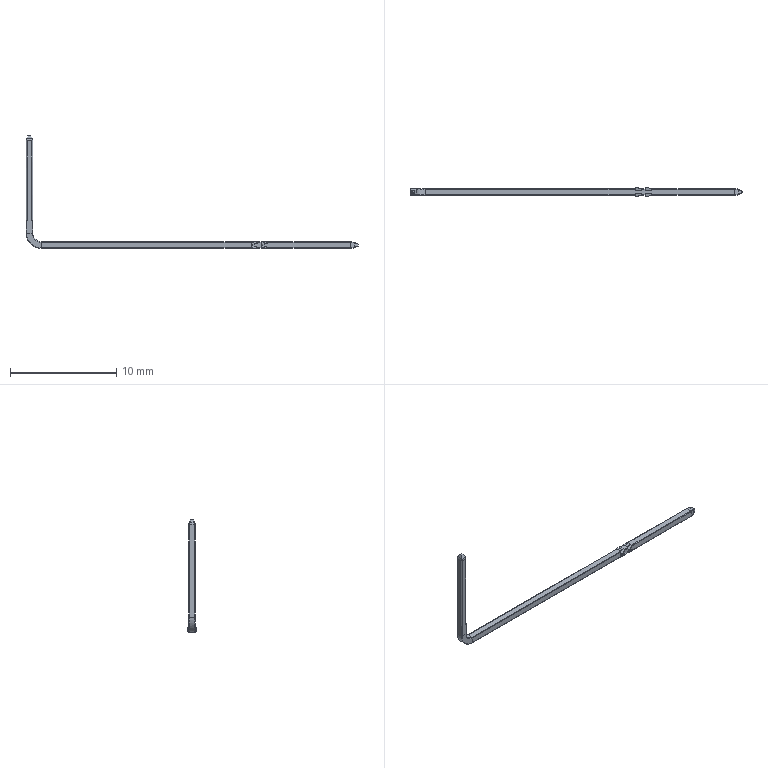Part | NX | features BREP 1 | 1 solid | 206 faces | box 31.215 x 0.8779 x 10.616 mm | volume 15.757 mm3 | cylinder 86 | plane 72 | torus 22 | sphere 20 | spline 6 | commonest cylinder face diameters 0.09 x28 0.1 x28 0.2 x12 2.01 x8 1 x4 2 x4